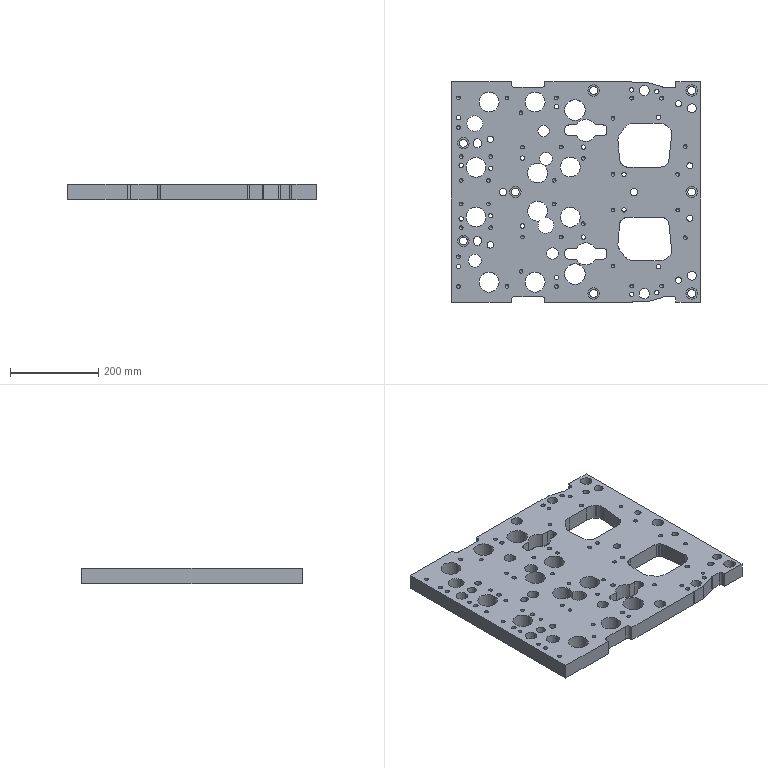Part | STEP file | 180_id4582_x_t | 1 solid | 259 faces | box 565 x 500 x 35 mm | volume 7605579 mm3 | cylinder 136 | plane 58 | cone 38 | spline 27 | commonest cylinder face diameters 8.506 x38 10 x26 20 x12 45 x10 18.009 x8 26.008 x8